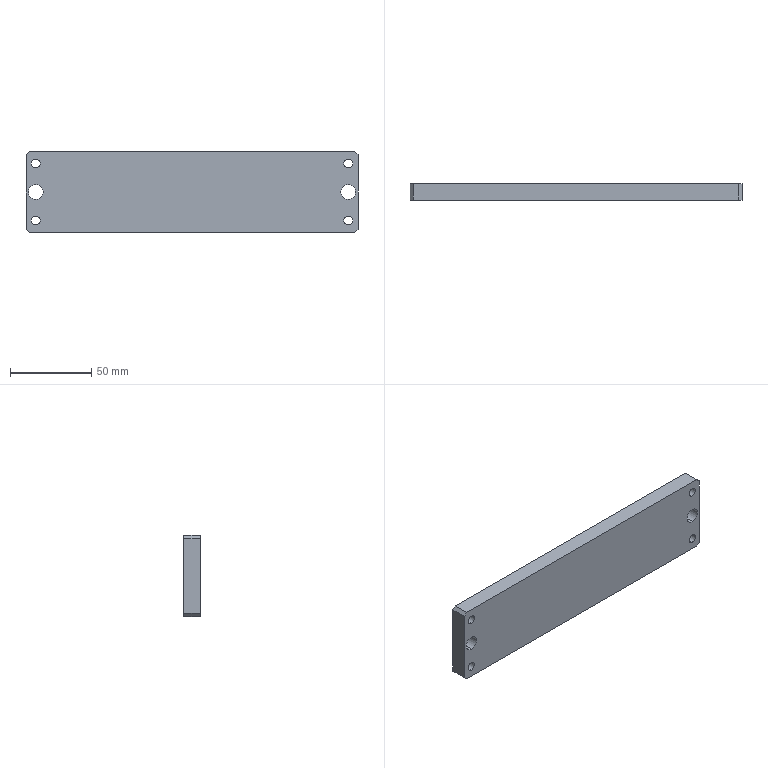Part | STEP file | MT-COMBO-119-S011 | 1 solid | 34 faces | box 204 x 10 x 50 mm | volume 98448 mm3 | cylinder 20 | plane 14 | commonest cylinder face diameters 5.5 x8 10 x8 9 x4
STEP:
#1=CARTESIAN_POINT('',(96.,-5.,-4.5));
#2=VERTEX_POINT('',#1);
#3=CARTESIAN_POINT('',(96.,-5.,4.5));
#4=VERTEX_POINT('',#3);
#5=CARTESIAN_POINT('',(96.,-5.,0.));
#6=DIRECTION('',(0.,-1.,0.));
#7=DIRECTION('',(0.,0.,-1.));
#8=AXIS2_PLACEMENT_3D('',#5,#6,#7);
#9=CIRCLE('',#8,4.5);
#10=EDGE_CURVE('',#2,#4,#9,.T.);
#11=ORIENTED_EDGE('',*,*,#10,.T.);
#12=CARTESIAN_POINT('',(96.,5.,4.5));
#13=VERTEX_POINT('',#12);
#14=CARTESIAN_POINT('',(96.,5.,4.5));
#15=DIRECTION('',(0.,1.,0.));
#16=VECTOR('',#15,1000.);
#17=LINE('',#14,#16);
#18=EDGE_CURVE('',#4,#13,#17,.T.);
#19=ORIENTED_EDGE('',*,*,#18,.T.);
#20=CARTESIAN_POINT('',(96.,5.,-4.5));
#21=VERTEX_POINT('',#20);
#22=CARTESIAN_POINT('',(96.,5.,0.));
#23=DIRECTION('',(0.,-1.,0.));
#24=DIRECTION('',(0.,0.,-1.));
#25=AXIS2_PLACEMENT_3D('',#22,#23,#24);
#26=CIRCLE('',#25,4.5);
#27=EDGE_CURVE('',#21,#13,#26,.T.);
#28=ORIENTED_EDGE('',*,*,#27,.F.);
#29=CARTESIAN_POINT('',(96.,5.,-4.5));
#30=DIRECTION('',(0.,1.,0.));
#31=VECTOR('',#30,1000.);
#32=LINE('',#29,#31);
#33=EDGE_CURVE('',#2,#21,#32,.T.);
#34=ORIENTED_EDGE('',*,*,#33,.F.);
#35=EDGE_LOOP('',(#11,#19,#28,#34));
#36=FACE_OUTER_BOUND('',#35,.T.);
#37=CARTESIAN_POINT('',(96.,5.,0.));
#38=DIRECTION('',(0.,1.,0.));
#39=DIRECTION('',(0.,0.,-1.));
#40=AXIS2_PLACEMENT_3D('',#37,#38,#39);
#41=CYLINDRICAL_SURFACE('',#40,4.5);
#42=ADVANCED_FACE('',(#36),#41,.F.);
#43=CARTESIAN_POINT('',(-96.,-5.,-4.5));
#44=VERTEX_POINT('',#43);
#45=CARTESIAN_POINT('',(-96.,-5.,4.5));
#46=VERTEX_POINT('',#45);
#47=CARTESIAN_POINT('',(-96.,-5.,0.));
#48=DIRECTION('',(0.,-1.,0.));
#49=DIRECTION('',(0.,0.,-1.));
#50=AXIS2_PLACEMENT_3D('',#47,#48,#49);
#51=CIRCLE('',#50,4.5);
#52=EDGE_CURVE('',#44,#46,#51,.T.);
#53=ORIENTED_EDGE('',*,*,#52,.T.);
#54=CARTESIAN_POINT('',(-96.,5.,4.5));
#55=VERTEX_POINT('',#54);
#56=CARTESIAN_POINT('',(-96.,5.,4.5));
#57=DIRECTION('',(0.,1.,0.));
#58=VECTOR('',#57,1000.);
#59=LINE('',#56,#58);
#60=EDGE_CURVE('',#46,#55,#59,.T.);
#61=ORIENTED_EDGE('',*,*,#60,.T.);
#62=CARTESIAN_POINT('',(-96.,5.,-4.5));
#63=VERTEX_POINT('',#62);
#64=CARTESIAN_POINT('',(-96.,5.,0.));
#65=DIRECTION('',(0.,-1.,0.));
#66=DIRECTION('',(0.,0.,-1.));
#67=AXIS2_PLACEMENT_3D('',#64,#65,#66);
#68=CIRCLE('',#67,4.5);
#69=EDGE_CURVE('',#63,#55,#68,.T.);
#70=ORIENTED_EDGE('',*,*,#69,.F.);
#71=CARTESIAN_POINT('',(-96.,5.,-4.5));
#72=DIRECTION('',(0.,1.,0.));
#73=VECTOR('',#72,1000.);
#74=LINE('',#71,#73);
#75=EDGE_CURVE('',#44,#63,#74,.T.);
#76=ORIENTED_EDGE('',*,*,#75,.F.);
#77=EDGE_LOOP('',(#53,#61,#70,#76));
#78=FACE_OUTER_BOUND('',#77,.T.);
#79=CARTESIAN_POINT('',(-96.,5.,0.));
#80=DIRECTION('',(0.,1.,0.));
#81=DIRECTION('',(0.,0.,-1.));
#82=AXIS2_PLACEMENT_3D('',#79,#80,#81);
#83=CYLINDRICAL_SURFACE('',#82,4.5);
#84=ADVANCED_FACE('',(#78),#83,.F.);
#85=CARTESIAN_POINT('',(-96.,-0.7,12.5));
#86=VERTEX_POINT('',#85);
#87=CARTESIAN_POINT('',(-96.,-0.7,22.5));
#88=VERTEX_POINT('',#87);
#89=CARTESIAN_POINT('',(-96.,-0.7,17.5));
#90=DIRECTION('',(0.,-1.,0.));
#91=DIRECTION('',(0.,0.,-1.));
#92=AXIS2_PLACEMENT_3D('',#89,#90,#91);
#93=CIRCLE('',#92,5.);
#94=EDGE_CURVE('',#86,#88,#93,.T.);
#95=ORIENTED_EDGE('',*,*,#94,.T.);
#96=CARTESIAN_POINT('',(-96.,5.,22.5));
#97=VERTEX_POINT('',#96);
#98=CARTESIAN_POINT('',(-96.,5.,22.5));
#99=DIRECTION('',(0.,1.,0.));
#100=VECTOR('',#99,1000.);
#101=LINE('',#98,#100);
#102=EDGE_CURVE('',#88,#97,#101,.T.);
#103=ORIENTED_EDGE('',*,*,#102,.T.);
#104=CARTESIAN_POINT('',(-96.,5.,12.5));
#105=VERTEX_POINT('',#104);
#106=CARTESIAN_POINT('',(-96.,5.,17.5));
#107=DIRECTION('',(0.,-1.,0.));
#108=DIRECTION('',(0.,0.,-1.));
#109=AXIS2_PLACEMENT_3D('',#106,#107,#108);
#110=CIRCLE('',#109,5.);
#111=EDGE_CURVE('',#105,#97,#110,.T.);
#112=ORIENTED_EDGE('',*,*,#111,.F.);
#113=CARTESIAN_POINT('',(-96.,5.,12.5));
#114=DIRECTION('',(0.,1.,0.));
#115=VECTOR('',#114,1000.);
#116=LINE('',#113,#115);
#117=EDGE_CURVE('',#86,#105,#116,.T.);
#118=ORIENTED_EDGE('',*,*,#117,.F.);
#119=EDGE_LOOP('',(#95,#103,#112,#118));
#120=FACE_OUTER_BOUND('',#119,.T.);
#121=CARTESIAN_POINT('',(-96.,5.,17.5));
#122=DIRECTION('',(0.,1.,0.));
#123=DIRECTION('',(0.,0.,-1.));
#124=AXIS2_PLACEMENT_3D('',#121,#122,#123);
#125=CYLINDRICAL_SURFACE('',#124,5.);
#126=ADVANCED_FACE('',(#120),#125,.F.);
#127=CARTESIAN_POINT('',(-96.,-5.,14.75));
#128=VERTEX_POINT('',#127);
#129=CARTESIAN_POINT('',(-96.,-5.,20.25));
#130=VERTEX_POINT('',#129);
#131=CARTESIAN_POINT('',(-96.,-5.,17.5));
#132=DIRECTION('',(0.,-1.,0.));
#133=DIRECTION('',(0.,0.,-1.));
#134=AXIS2_PLACEMENT_3D('',#131,#132,#133);
#135=CIRCLE('',#134,2.75);
#136=EDGE_CURVE('',#128,#130,#135,.T.);
#137=ORIENTED_EDGE('',*,*,#136,.T.);
#138=CARTESIAN_POINT('',(-96.,-0.7,20.25));
#139=VERTEX_POINT('',#138);
#140=CARTESIAN_POINT('',(-96.,5.,20.25));
#141=DIRECTION('',(0.,1.,0.));
#142=VECTOR('',#141,1000.);
#143=LINE('',#140,#142);
#144=EDGE_CURVE('',#130,#139,#143,.T.);
#145=ORIENTED_EDGE('',*,*,#144,.T.);
#146=CARTESIAN_POINT('',(-96.,-0.7,14.75));
#147=VERTEX_POINT('',#146);
#148=CARTESIAN_POINT('',(-96.,-0.7,17.5));
#149=DIRECTION('',(0.,-1.,0.));
#150=DIRECTION('',(0.,0.,-1.));
#151=AXIS2_PLACEMENT_3D('',#148,#149,#150);
#152=CIRCLE('',#151,2.75);
#153=EDGE_CURVE('',#147,#139,#152,.T.);
#154=ORIENTED_EDGE('',*,*,#153,.F.);
#155=CARTESIAN_POINT('',(-96.,5.,14.75));
#156=DIRECTION('',(0.,1.,0.));
#157=VECTOR('',#156,1000.);
#158=LINE('',#155,#157);
#159=EDGE_CURVE('',#128,#147,#158,.T.);
#160=ORIENTED_EDGE('',*,*,#159,.F.);
#161=EDGE_LOOP('',(#137,#145,#154,#160));
#162=FACE_OUTER_BOUND('',#161,.T.);
#163=CARTESIAN_POINT('',(-96.,5.,17.5));
#164=DIRECTION('',(0.,1.,0.));
#165=DIRECTION('',(0.,0.,-1.));
#166=AXIS2_PLACEMENT_3D('',#163,#164,#165);
#167=CYLINDRICAL_SURFACE('',#166,2.75);
#168=ADVANCED_FACE('',(#162),#167,.F.);
#169=CARTESIAN_POINT('',(-96.,-0.7,-22.5));
#170=VERTEX_POINT('',#169);
#171=CARTESIAN_POINT('',(-96.,-0.7,-12.5));
#172=VERTEX_POINT('',#171);
#173=CARTESIAN_POINT('',(-96.,-0.7,-17.5));
#174=DIRECTION('',(0.,-1.,0.));
#175=DIRECTION('',(0.,0.,-1.));
#176=AXIS2_PLACEMENT_3D('',#173,#174,#175);
#177=CIRCLE('',#176,5.);
#178=EDGE_CURVE('',#170,#172,#177,.T.);
#179=ORIENTED_EDGE('',*,*,#178,.T.);
#180=CARTESIAN_POINT('',(-96.,5.,-12.5));
#181=VERTEX_POINT('',#180);
#182=CARTESIAN_POINT('',(-96.,5.,-12.5));
#183=DIRECTION('',(0.,1.,0.));
#184=VECTOR('',#183,1000.);
#185=LINE('',#182,#184);
#186=EDGE_CURVE('',#172,#181,#185,.T.);
#187=ORIENTED_EDGE('',*,*,#186,.T.);
#188=CARTESIAN_POINT('',(-96.,5.,-22.5));
#189=VERTEX_POINT('',#188);
#190=CARTESIAN_POINT('',(-96.,5.,-17.5));
#191=DIRECTION('',(0.,-1.,0.));
#192=DIRECTION('',(0.,0.,-1.));
#193=AXIS2_PLACEMENT_3D('',#190,#191,#192);
#194=CIRCLE('',#193,5.);
#195=EDGE_CURVE('',#189,#181,#194,.T.);
#196=ORIENTED_EDGE('',*,*,#195,.F.);
#197=CARTESIAN_POINT('',(-96.,5.,-22.5));
#198=DIRECTION('',(0.,1.,0.));
#199=VECTOR('',#198,1000.);
#200=LINE('',#197,#199);
#201=EDGE_CURVE('',#170,#189,#200,.T.);
#202=ORIENTED_EDGE('',*,*,#201,.F.);
#203=EDGE_LOOP('',(#179,#187,#196,#202));
#204=FACE_OUTER_BOUND('',#203,.T.);
#205=CARTESIAN_POINT('',(-96.,5.,-17.5));
#206=DIRECTION('',(0.,1.,0.));
#207=DIRECTION('',(0.,0.,-1.));
#208=AXIS2_PLACEMENT_3D('',#205,#206,#207);
#209=CYLINDRICAL_SURFACE('',#208,5.);
#210=ADVANCED_FACE('',(#204),#209,.F.);
#211=CARTESIAN_POINT('',(-96.,-5.,-20.25));
#212=VERTEX_POINT('',#211);
#213=CARTESIAN_POINT('',(-96.,-5.,-14.75));
#214=VERTEX_POINT('',#213);
#215=CARTESIAN_POINT('',(-96.,-5.,-17.5));
#216=DIRECTION('',(0.,-1.,0.));
#217=DIRECTION('',(0.,0.,-1.));
#218=AXIS2_PLACEMENT_3D('',#215,#216,#217);
#219=CIRCLE('',#218,2.75);
#220=EDGE_CURVE('',#212,#214,#219,.T.);
#221=ORIENTED_EDGE('',*,*,#220,.T.);
#222=CARTESIAN_POINT('',(-96.,-0.7,-14.75));
#223=VERTEX_POINT('',#222);
#224=CARTESIAN_POINT('',(-96.,5.,-14.75));
#225=DIRECTION('',(0.,1.,0.));
#226=VECTOR('',#225,1000.);
#227=LINE('',#224,#226);
#228=EDGE_CURVE('',#214,#223,#227,.T.);
#229=ORIENTED_EDGE('',*,*,#228,.T.);
#230=CARTESIAN_POINT('',(-96.,-0.7,-20.25));
#231=VERTEX_POINT('',#230);
#232=CARTESIAN_POINT('',(-96.,-0.7,-17.5));
#233=DIRECTION('',(0.,-1.,0.));
#234=DIRECTION('',(0.,0.,-1.));
#235=AXIS2_PLACEMENT_3D('',#232,#233,#234);
#236=CIRCLE('',#235,2.75);
#237=EDGE_CURVE('',#231,#223,#236,.T.);
#238=ORIENTED_EDGE('',*,*,#237,.F.);
#239=CARTESIAN_POINT('',(-96.,5.,-20.25));
#240=DIRECTION('',(0.,1.,0.));
#241=VECTOR('',#240,1000.);
#242=LINE('',#239,#241);
#243=EDGE_CURVE('',#212,#231,#242,.T.);
#244=ORIENTED_EDGE('',*,*,#243,.F.);
#245=EDGE_LOOP('',(#221,#229,#238,#244));
#246=FACE_OUTER_BOUND('',#245,.T.);
#247=CARTESIAN_POINT('',(-96.,5.,-17.5));
#248=DIRECTION('',(0.,1.,0.));
#249=DIRECTION('',(0.,0.,-1.));
#250=AXIS2_PLACEMENT_3D('',#247,#248,#249);
#251=CYLINDRICAL_SURFACE('',#250,2.75);
#252=ADVANCED_FACE('',(#246),#251,.F.);
#253=CARTESIAN_POINT('',(96.,-0.7,-22.5));
#254=VERTEX_POINT('',#253);
#255=CARTESIAN_POINT('',(96.,-0.7,-12.5));
#256=VERTEX_POINT('',#255);
#257=CARTESIAN_POINT('',(96.,-0.7,-17.5));
#258=DIRECTION('',(0.,-1.,0.));
#259=DIRECTION('',(0.,0.,-1.));
#260=AXIS2_PLACEMENT_3D('',#257,#258,#259);
#261=CIRCLE('',#260,5.);
#262=EDGE_CURVE('',#254,#256,#261,.T.);
#263=ORIENTED_EDGE('',*,*,#262,.T.);
#264=CARTESIAN_POINT('',(96.,5.,-12.5));
#265=VERTEX_POINT('',#264);
#266=CARTESIAN_POINT('',(96.,5.,-12.5));
#267=DIRECTION('',(0.,1.,0.));
#268=VECTOR('',#267,1000.);
#269=LINE('',#266,#268);
#270=EDGE_CURVE('',#256,#265,#269,.T.);
#271=ORIENTED_EDGE('',*,*,#270,.T.);
#272=CARTESIAN_POINT('',(96.,5.,-22.5));
#273=VERTEX_POINT('',#272);
#274=CARTESIAN_POINT('',(96.,5.,-17.5));
#275=DIRECTION('',(0.,-1.,0.));
#276=DIRECTION('',(0.,0.,-1.));
#277=AXIS2_PLACEMENT_3D('',#274,#275,#276);
#278=CIRCLE('',#277,5.);
#279=EDGE_CURVE('',#273,#265,#278,.T.);
#280=ORIENTED_EDGE('',*,*,#279,.F.);
#281=CARTESIAN_POINT('',(96.,5.,-22.5));
#282=DIRECTION('',(0.,1.,0.));
#283=VECTOR('',#282,1000.);
#284=LINE('',#281,#283);
#285=EDGE_CURVE('',#254,#273,#284,.T.);
#286=ORIENTED_EDGE('',*,*,#285,.F.);
#287=EDGE_LOOP('',(#263,#271,#280,#286));
#288=FACE_OUTER_BOUND('',#287,.T.);
#289=CARTESIAN_POINT('',(96.,5.,-17.5));
#290=DIRECTION('',(0.,1.,0.));
#291=DIRECTION('',(0.,0.,-1.));
#292=AXIS2_PLACEMENT_3D('',#289,#290,#291);
#293=CYLINDRICAL_SURFACE('',#292,5.);
#294=ADVANCED_FACE('',(#288),#293,.F.);
#295=CARTESIAN_POINT('',(96.,-5.,-20.25));
#296=VERTEX_POINT('',#295);
#297=CARTESIAN_POINT('',(96.,-5.,-14.75));
#298=VERTEX_POINT('',#297);
#299=CARTESIAN_POINT('',(96.,-5.,-17.5));
#300=DIRECTION('',(0.,-1.,0.));
#301=DIRECTION('',(0.,0.,-1.));
#302=AXIS2_PLACEMENT_3D('',#299,#300,#301);
#303=CIRCLE('',#302,2.75);
#304=EDGE_CURVE('',#296,#298,#303,.T.);
#305=ORIENTED_EDGE('',*,*,#304,.T.);
#306=CARTESIAN_POINT('',(96.,-0.7,-14.75));
#307=VERTEX_POINT('',#306);
#308=CARTESIAN_POINT('',(96.,5.,-14.75));
#309=DIRECTION('',(0.,1.,0.));
#310=VECTOR('',#309,1000.);
#311=LINE('',#308,#310);
#312=EDGE_CURVE('',#298,#307,#311,.T.);
#313=ORIENTED_EDGE('',*,*,#312,.T.);
#314=CARTESIAN_POINT('',(96.,-0.7,-20.25));
#315=VERTEX_POINT('',#314);
#316=CARTESIAN_POINT('',(96.,-0.7,-17.5));
#317=DIRECTION('',(0.,-1.,0.));
#318=DIRECTION('',(0.,0.,-1.));
#319=AXIS2_PLACEMENT_3D('',#316,#317,#318);
#320=CIRCLE('',#319,2.75);
#321=EDGE_CURVE('',#315,#307,#320,.T.);
#322=ORIENTED_EDGE('',*,*,#321,.F.);
#323=CARTESIAN_POINT('',(96.,5.,-20.25));
#324=DIRECTION('',(0.,1.,0.));
#325=VECTOR('',#324,1000.);
#326=LINE('',#323,#325);
#327=EDGE_CURVE('',#296,#315,#326,.T.);
#328=ORIENTED_EDGE('',*,*,#327,.F.);
#329=EDGE_LOOP('',(#305,#313,#322,#328));
#330=FACE_OUTER_BOUND('',#329,.T.);
#331=CARTESIAN_POINT('',(96.,5.,-17.5));
#332=DIRECTION('',(0.,1.,0.));
#333=DIRECTION('',(0.,0.,-1.));
#334=AXIS2_PLACEMENT_3D('',#331,#332,#333);
#335=CYLINDRICAL_SURFACE('',#334,2.75);
#336=ADVANCED_FACE('',(#330),#335,.F.);
#337=CARTESIAN_POINT('',(96.,-0.7,12.5));
#338=VERTEX_POINT('',#337);
#339=CARTESIAN_POINT('',(96.,-0.7,22.5));
#340=VERTEX_POINT('',#339);
#341=CARTESIAN_POINT('',(96.,-0.7,17.5));
#342=DIRECTION('',(0.,-1.,0.));
#343=DIRECTION('',(0.,0.,-1.));
#344=AXIS2_PLACEMENT_3D('',#341,#342,#343);
#345=CIRCLE('',#344,5.);
#346=EDGE_CURVE('',#338,#340,#345,.T.);
#347=ORIENTED_EDGE('',*,*,#346,.T.);
#348=CARTESIAN_POINT('',(96.,5.,22.5));
#349=VERTEX_POINT('',#348);
#350=CARTESIAN_POINT('',(96.,5.,22.5));
#351=DIRECTION('',(0.,1.,0.));
#352=VECTOR('',#351,1000.);
#353=LINE('',#350,#352);
#354=EDGE_CURVE('',#340,#349,#353,.T.);
#355=ORIENTED_EDGE('',*,*,#354,.T.);
#356=CARTESIAN_POINT('',(96.,5.,12.5));
#357=VERTEX_POINT('',#356);
#358=CARTESIAN_POINT('',(96.,5.,17.5));
#359=DIRECTION('',(0.,-1.,0.));
#360=DIRECTION('',(0.,0.,-1.));
#361=AXIS2_PLACEMENT_3D('',#358,#359,#360);
#362=CIRCLE('',#361,5.);
#363=EDGE_CURVE('',#357,#349,#362,.T.);
#364=ORIENTED_EDGE('',*,*,#363,.F.);
#365=CARTESIAN_POINT('',(96.,5.,12.5));
#366=DIRECTION('',(0.,1.,0.));
#367=VECTOR('',#366,1000.);
#368=LINE('',#365,#367);
#369=EDGE_CURVE('',#338,#357,#368,.T.);
#370=ORIENTED_EDGE('',*,*,#369,.F.);
#371=EDGE_LOOP('',(#347,#355,#364,#370));
#372=FACE_OUTER_BOUND('',#371,.T.);
#373=CARTESIAN_POINT('',(96.,5.,17.5));
#374=DIRECTION('',(0.,1.,0.));
#375=DIRECTION('',(0.,0.,-1.));
#376=AXIS2_PLACEMENT_3D('',#373,#374,#375);
#377=CYLINDRICAL_SURFACE('',#376,5.);
#378=ADVANCED_FACE('',(#372),#377,.F.);
#379=CARTESIAN_POINT('',(96.,-5.,14.75));
#380=VERTEX_POINT('',#379);
#381=CARTESIAN_POINT('',(96.,-5.,20.25));
#382=VERTEX_POINT('',#381);
#383=CARTESIAN_POINT('',(96.,-5.,17.5));
#384=DIRECTION('',(0.,-1.,0.));
#385=DIRECTION('',(0.,0.,-1.));
#386=AXIS2_PLACEMENT_3D('',#383,#384,#385);
#387=CIRCLE('',#386,2.75);
#388=EDGE_CURVE('',#380,#382,#387,.T.);
#389=ORIENTED_EDGE('',*,*,#388,.T.);
#390=CARTESIAN_POINT('',(96.,-0.7,20.25));
#391=VERTEX_POINT('',#390);
#392=CARTESIAN_POINT('',(96.,5.,20.25));
#393=DIRECTION('',(0.,1.,0.));
#394=VECTOR('',#393,1000.);
#395=LINE('',#392,#394);
#396=EDGE_CURVE('',#382,#391,#395,.T.);
#397=ORIENTED_EDGE('',*,*,#396,.T.);
#398=CARTESIAN_POINT('',(96.,-0.7,14.75));
#399=VERTEX_POINT('',#398);
#400=CARTESIAN_POINT('',(96.,-0.7,17.5));
#401=DIRECTION('',(0.,-1.,0.));
#402=DIRECTION('',(0.,0.,-1.));
#403=AXIS2_PLACEMENT_3D('',#400,#401,#402);
#404=CIRCLE('',#403,2.75);
#405=EDGE_CURVE('',#399,#391,#404,.T.);
#406=ORIENTED_EDGE('',*,*,#405,.F.);
#407=CARTESIAN_POINT('',(96.,5.,14.75));
#408=DIRECTION('',(0.,1.,0.));
#409=VECTOR('',#408,1000.);
#410=LINE('',#407,#409);
#411=EDGE_CURVE('',#380,#399,#410,.T.);
#412=ORIENTED_EDGE('',*,*,#411,.F.);
#413=EDGE_LOOP('',(#389,#397,#406,#412));
#414=FACE_OUTER_BOUND('',#413,.T.);
#415=CARTESIAN_POINT('',(96.,5.,17.5));
#416=DIRECTION('',(0.,1.,0.));
#417=DIRECTION('',(0.,0.,-1.));
#418=AXIS2_PLACEMENT_3D('',#415,#416,#417);
#419=CYLINDRICAL_SURFACE('',#418,2.75);
#420=ADVANCED_FACE('',(#414),#419,.F.);
#421=CARTESIAN_POINT('',(102.,-5.,-23.));
#422=VERTEX_POINT('',#421);
#423=CARTESIAN_POINT('',(102.,-5.,23.));
#424=VERTEX_POINT('',#423);
#425=CARTESIAN_POINT('',(102.,-5.,25.));
#426=DIRECTION('',(0.,0.,1.));
#427=VECTOR('',#426,1000.);
#428=LINE('',#425,#427);
#429=EDGE_CURVE('',#422,#424,#428,.T.);
#430=ORIENTED_EDGE('',*,*,#429,.F.);
#431=CARTESIAN_POINT('',(102.,5.,-23.));
#432=VERTEX_POINT('',#431);
#433=CARTESIAN_POINT('',(102.,5.,-23.));
#434=DIRECTION('',(0.,-1.,0.));
#435=VECTOR('',#434,1000.);
#436=LINE('',#433,#435);
#437=EDGE_CURVE('',#432,#422,#436,.T.);
#438=ORIENTED_EDGE('',*,*,#437,.F.);
#439=CARTESIAN_POINT('',(102.,5.,23.));
#440=VERTEX_POINT('',#439);
#441=CARTESIAN_POINT('',(102.,5.,25.));
#442=DIRECTION('',(0.,0.,1.));
#443=VECTOR('',#442,1000.);
#444=LINE('',#441,#443);
#445=EDGE_CURVE('',#432,#440,#444,.T.);
#446=ORIENTED_EDGE('',*,*,#445,.T.);
#447=CARTESIAN_POINT('',(102.,5.,23.));
#448=DIRECTION('',(0.,1.,0.));
#449=VECTOR('',#448,1000.);
#450=LINE('',#447,#449);
#451=EDGE_CURVE('',#424,#440,#450,.T.);
#452=ORIENTED_EDGE('',*,*,#451,.F.);
#453=EDGE_LOOP('',(#430,#438,#446,#452));
#454=FACE_OUTER_BOUND('',#453,.T.);
#455=CARTESIAN_POINT('',(102.,5.,25.));
#456=DIRECTION('',(-1.,0.,0.));
#457=DIRECTION('',(0.,0.,-1.));
#458=AXIS2_PLACEMENT_3D('',#455,#456,#457);
#459=PLANE('',#458);
#460=ADVANCED_FACE('',(#454),#459,.F.);
#461=CARTESIAN_POINT('',(100.,5.,25.));
#462=VERTEX_POINT('',#461);
#463=CARTESIAN_POINT('',(-100.,5.,25.));
#464=VERTEX_POINT('',#463);
#465=CARTESIAN_POINT('',(-154.5,5.,25.));
#466=DIRECTION('',(-1.,0.,0.));
#467=VECTOR('',#466,1000.);
#468=LINE('',#465,#467);
#469=EDGE_CURVE('',#462,#464,#468,.T.);
#470=ORIENTED_EDGE('',*,*,#469,.T.);
#471=CARTESIAN_POINT('',(-100.,-5.,25.));
#472=VERTEX_POINT('',#471);
#473=CARTESIAN_POINT('',(-100.,5.,25.));
#474=DIRECTION('',(0.,1.,0.));
#475=VECTOR('',#474,1000.);
#476=LINE('',#473,#475);
#477=EDGE_CURVE('',#472,#464,#476,.T.);
#478=ORIENTED_EDGE('',*,*,#477,.F.);
#479=CARTESIAN_POINT('',(100.,-5.,25.));
#480=VERTEX_POINT('',#479);
#481=CARTESIAN_POINT('',(-154.5,-5.,25.));
#482=DIRECTION('',(-1.,0.,0.));
#483=VECTOR('',#482,1000.);
#484=LINE('',#481,#483);
#485=EDGE_CURVE('',#480,#472,#484,.T.);
#486=ORIENTED_EDGE('',*,*,#485,.F.);
#487=CARTESIAN_POINT('',(100.,5.,25.));
#488=DIRECTION('',(0.,-1.,0.));
#489=VECTOR('',#488,1000.);
#490=LINE('',#487,#489);
#491=EDGE_CURVE('',#462,#480,#490,.T.);
#492=ORIENTED_EDGE('',*,*,#491,.F.);
#493=EDGE_LOOP('',(#470,#478,#486,#492));
#494=FACE_OUTER_BOUND('',#493,.T.);
#495=CARTESIAN_POINT('',(-154.5,5.,25.));
#496=DIRECTION('',(0.,0.,-1.));
#497=DIRECTION('',(1.,0.,0.));
#498=AXIS2_PLACEMENT_3D('',#495,#496,#497);
#499=PLANE('',#498);
#500=ADVANCED_FACE('',(#494),#499,.F.);
#501=CARTESIAN_POINT('',(-102.,5.,23.));
#502=VERTEX_POINT('',#501);
#503=CARTESIAN_POINT('',(-102.,5.,-23.));
#504=VERTEX_POINT('',#503);
#505=CARTESIAN_POINT('',(-102.,5.,25.));
#506=DIRECTION('',(0.,0.,-1.));
#507=VECTOR('',#506,1000.);
#508=LINE('',#505,#507);
#509=EDGE_CURVE('',#502,#504,#508,.T.);
#510=ORIENTED_EDGE('',*,*,#509,.T.);
#511=CARTESIAN_POINT('',(-102.,-5.,-23.));
#512=VERTEX_POINT('',#511);
#513=CARTESIAN_POINT('',(-102.,5.,-23.));
#514=DIRECTION('',(0.,1.,0.));
#515=VECTOR('',#514,1000.);
#516=LINE('',#513,#515);
#517=EDGE_CURVE('',#512,#504,#516,.T.);
#518=ORIENTED_EDGE('',*,*,#517,.F.);
#519=CARTESIAN_POINT('',(-102.,-5.,23.));
#520=VERTEX_POINT('',#519);
#521=CARTESIAN_POINT('',(-102.,-5.,25.));
#522=DIRECTION('',(0.,0.,-1.));
#523=VECTOR('',#522,1000.);
#524=LINE('',#521,#523);
#525=EDGE_CURVE('',#520,#512,#524,.T.);
#526=ORIENTED_EDGE('',*,*,#525,.F.);
#527=CARTESIAN_POINT('',(-102.,5.,23.));
#528=DIRECTION('',(0.,-1.,0.));
#529=VECTOR('',#528,1000.);
#530=LINE('',#527,#529);
#531=EDGE_CURVE('',#502,#520,#530,.T.);
#532=ORIENTED_EDGE('',*,*,#531,.F.);
#533=EDGE_LOOP('',(#510,#518,#526,#532));
#534=FACE_OUTER_BOUND('',#533,.T.);
#535=CARTESIAN_POINT('',(-102.,5.,25.));
#536=DIRECTION('',(1.,0.,0.));
#537=DIRECTION('',(0.,0.,1.));
#538=AXIS2_PLACEMENT_3D('',#535,#536,#537);
#539=PLANE('',#538);
#540=ADVANCED_FACE('',(#534),#539,.F.);
#541=CARTESIAN_POINT('',(-100.,-5.,-25.));
#542=VERTEX_POINT('',#541);
#543=CARTESIAN_POINT('',(100.,-5.,-25.));
#544=VERTEX_POINT('',#543);
#545=CARTESIAN_POINT('',(-154.5,-5.,-25.));
#546=DIRECTION('',(1.,0.,0.));
#547=VECTOR('',#546,1000.);
#548=LINE('',#545,#547);
#549=EDGE_CURVE('',#542,#544,#548,.T.);
#550=ORIENTED_EDGE('',*,*,#549,.F.);
#551=CARTESIAN_POINT('',(-100.,5.,-25.));
#552=VERTEX_POINT('',#551);
#553=CARTESIAN_POINT('',(-100.,5.,-25.));
#554=DIRECTION('',(0.,-1.,0.));
#555=VECTOR('',#554,1000.);
#556=LINE('',#553,#555);
#557=EDGE_CURVE('',#552,#542,#556,.T.);
#558=ORIENTED_EDGE('',*,*,#557,.F.);
#559=CARTESIAN_POINT('',(100.,5.,-25.));
#560=VERTEX_POINT('',#559);
#561=CARTESIAN_POINT('',(-154.5,5.,-25.));
#562=DIRECTION('',(1.,0.,0.));
#563=VECTOR('',#562,1000.);
#564=LINE('',#561,#563);
#565=EDGE_CURVE('',#552,#560,#564,.T.);
#566=ORIENTED_EDGE('',*,*,#565,.T.);
#567=CARTESIAN_POINT('',(100.,5.,-25.));
#568=DIRECTION('',(0.,1.,0.));
#569=VECTOR('',#568,1000.);
#570=LINE('',#567,#569);
#571=EDGE_CURVE('',#544,#560,#570,.T.);
#572=ORIENTED_EDGE('',*,*,#571,.F.);
#573=EDGE_LOOP('',(#550,#558,#566,#572));
#574=FACE_OUTER_BOUND('',#573,.T.);
#575=CARTESIAN_POINT('',(-154.5,5.,-25.));
#576=DIRECTION('',(0.,0.,1.));
#577=DIRECTION('',(-1.,0.,0.));
#578=AXIS2_PLACEMENT_3D('',#575,#576,#577);
#579=PLANE('',#578);
#580=ADVANCED_FACE('',(#574),#579,.F.);
#581=ORIENTED_EDGE('',*,*,#27,.T.);
#582=CARTESIAN_POINT('',(96.,5.,0.));
#583=DIRECTION('',(0.,-1.,0.));
#584=DIRECTION('',(0.,0.,-1.));
#585=AXIS2_PLACEMENT_3D('',#582,#583,#584);
#586=CIRCLE('',#585,4.5);
#587=EDGE_CURVE('',#13,#21,#586,.T.);
#588=ORIENTED_EDGE('',*,*,#587,.T.);
#589=EDGE_LOOP('',(#581,#588));
#590=FACE_BOUND('',#589,.T.);
#591=ORIENTED_EDGE('',*,*,#69,.T.);
#592=CARTESIAN_POINT('',(-96.,5.,0.));
#593=DIRECTION('',(0.,-1.,0.));
#594=DIRECTION('',(0.,0.,-1.));
#595=AXIS2_PLACEMENT_3D('',#592,#593,#594);
#596=CIRCLE('',#595,4.5);
#597=EDGE_CURVE('',#55,#63,#596,.T.);
#598=ORIENTED_EDGE('',*,*,#597,.T.);
#599=EDGE_LOOP('',(#591,#598));
#600=FACE_BOUND('',#599,.T.);
#601=ORIENTED_EDGE('',*,*,#111,.T.);
#602=CARTESIAN_POINT('',(-96.,5.,17.5));
#603=DIRECTION('',(0.,-1.,0.));
#604=DIRECTION('',(0.,0.,-1.));
#605=AXIS2_PLACEMENT_3D('',#602,#603,#604);
#606=CIRCLE('',#605,5.);
#607=EDGE_CURVE('',#97,#105,#606,.T.);
#608=ORIENTED_EDGE('',*,*,#607,.T.);
#609=EDGE_LOOP('',(#601,#608));
#610=FACE_BOUND('',#609,.T.);
#611=ORIENTED_EDGE('',*,*,#195,.T.);
#612=CARTESIAN_POINT('',(-96.,5.,-17.5));
#613=DIRECTION('',(0.,-1.,0.));
#614=DIRECTION('',(0.,0.,-1.));
#615=AXIS2_PLACEMENT_3D('',#612,#613,#614);
#616=CIRCLE('',#615,5.);
#617=EDGE_CURVE('',#181,#189,#616,.T.);
#618=ORIENTED_EDGE('',*,*,#617,.T.);
#619=EDGE_LOOP('',(#611,#618));
#620=FACE_BOUND('',#619,.T.);
#621=ORIENTED_EDGE('',*,*,#279,.T.);
#622=CARTESIAN_POINT('',(96.,5.,-17.5));
#623=DIRECTION('',(0.,-1.,0.));
#624=DIRECTION('',(0.,0.,-1.));
#625=AXIS2_PLACEMENT_3D('',#622,#623,#624);
#626=CIRCLE('',#625,5.);
#627=EDGE_CURVE('',#265,#273,#626,.T.);
#628=ORIENTED_EDGE('',*,*,#627,.T.);
#629=EDGE_LOOP('',(#621,#628));
#630=FACE_BOUND('',#629,.T.);
#631=ORIENTED_EDGE('',*,*,#363,.T.);
#632=CARTESIAN_POINT('',(96.,5.,17.5));
#633=DIRECTION('',(0.,-1.,0.));
#634=DIRECTION('',(0.,0.,-1.));
#635=AXIS2_PLACEMENT_3D('',#632,#633,#634);
#636=CIRCLE('',#635,5.);
#637=EDGE_CURVE('',#349,#357,#636,.T.);
#638=ORIENTED_EDGE('',*,*,#637,.T.);
#639=EDGE_LOOP('',(#631,#638));
#640=FACE_BOUND('',#639,.T.);
#641=ORIENTED_EDGE('',*,*,#445,.F.);
#642=CARTESIAN_POINT('',(36.25,5.,-88.75));
#643=DIRECTION('',(0.7071,0.,0.7071));
#644=VECTOR('',#643,1000.);
#645=LINE('',#642,#644);
#646=EDGE_CURVE('',#560,#432,#645,.T.);
#647=ORIENTED_EDGE('',*,*,#646,.F.);
#648=ORIENTED_EDGE('',*,*,#565,.F.);
#649=CARTESIAN_POINT('',(-36.25,5.,-88.75));
#650=DIRECTION('',(0.7071,0.,-0.7071));
#651=VECTOR('',#650,1000.);
#652=LINE('',#649,#651);
#653=EDGE_CURVE('',#504,#552,#652,.T.);
#654=ORIENTED_EDGE('',*,*,#653,.F.);
#655=ORIENTED_EDGE('',*,*,#509,.F.);
#656=CARTESIAN_POINT('',(-36.25,5.,88.75));
#657=DIRECTION('',(-0.7071,0.,-0.7071));
#658=VECTOR('',#657,1000.);
#659=LINE('',#656,#658);
#660=EDGE_CURVE('',#464,#502,#659,.T.);
#661=ORIENTED_EDGE('',*,*,#660,.F.);
#662=ORIENTED_EDGE('',*,*,#469,.F.);
#663=CARTESIAN_POINT('',(36.25,5.,88.75));
#664=DIRECTION('',(-0.7071,0.,0.7071));
#665=VECTOR('',#664,1000.);
#666=LINE('',#663,#665);
#667=EDGE_CURVE('',#440,#462,#666,.T.);
#668=ORIENTED_EDGE('',*,*,#667,.F.);
#669=EDGE_LOOP('',(#641,#647,#648,#654,#655,#661,#662,#668));
#670=FACE_OUTER_BOUND('',#669,.T.);
#671=CARTESIAN_POINT('',(0.,5.,0.));
#672=DIRECTION('',(0.,1.,0.));
#673=DIRECTION('',(0.,0.,-1.));
#674=AXIS2_PLACEMENT_3D('',#671,#672,#673);
#675=PLANE('',#674);
#676=ADVANCED_FACE('',(#590,#600,#610,#620,#630,#640,#670),#675,.T.);
#677=ORIENTED_EDGE('',*,*,#10,.F.);
#678=CARTESIAN_POINT('',(96.,-5.,0.));
#679=DIRECTION('',(0.,-1.,0.));
#680=DIRECTION('',(0.,0.,-1.));
#681=AXIS2_PLACEMENT_3D('',#678,#679,#680);
#682=CIRCLE('',#681,4.5);
#683=EDGE_CURVE('',#4,#2,#682,.T.);
#684=ORIENTED_EDGE('',*,*,#683,.F.);
#685=EDGE_LOOP('',(#677,#684));
#686=FACE_BOUND('',#685,.T.);
#687=ORIENTED_EDGE('',*,*,#52,.F.);
#688=CARTESIAN_POINT('',(-96.,-5.,0.));
#689=DIRECTION('',(0.,-1.,0.));
#690=DIRECTION('',(0.,0.,-1.));
#691=AXIS2_PLACEMENT_3D('',#688,#689,#690);
#692=CIRCLE('',#691,4.5);
#693=EDGE_CURVE('',#46,#44,#692,.T.);
#694=ORIENTED_EDGE('',*,*,#693,.F.);
#695=EDGE_LOOP('',(#687,#694));
#696=FACE_BOUND('',#695,.T.);
#697=ORIENTED_EDGE('',*,*,#136,.F.);
#698=CARTESIAN_POINT('',(-96.,-5.,17.5));
#699=DIRECTION('',(0.,-1.,0.));
#700=DIRECTION('',(0.,0.,-1.));
#701=AXIS2_PLACEMENT_3D('',#698,#699,#700);
#702=CIRCLE('',#701,2.75);
#703=EDGE_CURVE('',#130,#128,#702,.T.);
#704=ORIENTED_EDGE('',*,*,#703,.F.);
#705=EDGE_LOOP('',(#697,#704));
#706=FACE_BOUND('',#705,.T.);
#707=ORIENTED_EDGE('',*,*,#220,.F.);
#708=CARTESIAN_POINT('',(-96.,-5.,-17.5));
#709=DIRECTION('',(0.,-1.,0.));
#710=DIRECTION('',(0.,0.,-1.));
#711=AXIS2_PLACEMENT_3D('',#708,#709,#710);
#712=CIRCLE('',#711,2.75);
#713=EDGE_CURVE('',#214,#212,#712,.T.);
#714=ORIENTED_EDGE('',*,*,#713,.F.);
#715=EDGE_LOOP('',(#707,#714));
#716=FACE_BOUND('',#715,.T.);
#717=ORIENTED_EDGE('',*,*,#304,.F.);
#718=CARTESIAN_POINT('',(96.,-5.,-17.5));
#719=DIRECTION('',(0.,-1.,0.));
#720=DIRECTION('',(0.,0.,-1.));
#721=AXIS2_PLACEMENT_3D('',#718,#719,#720);
#722=CIRCLE('',#721,2.75);
#723=EDGE_CURVE('',#298,#296,#722,.T.);
#724=ORIENTED_EDGE('',*,*,#723,.F.);
#725=EDGE_LOOP('',(#717,#724));
#726=FACE_BOUND('',#725,.T.);
#727=ORIENTED_EDGE('',*,*,#388,.F.);
#728=CARTESIAN_POINT('',(96.,-5.,17.5));
#729=DIRECTION('',(0.,-1.,0.));
#730=DIRECTION('',(0.,0.,-1.));
#731=AXIS2_PLACEMENT_3D('',#728,#729,#730);
#732=CIRCLE('',#731,2.75);
#733=EDGE_CURVE('',#382,#380,#732,.T.);
#734=ORIENTED_EDGE('',*,*,#733,.F.);
#735=EDGE_LOOP('',(#727,#734));
#736=FACE_BOUND('',#735,.T.);
#737=ORIENTED_EDGE('',*,*,#485,.T.);
#738=CARTESIAN_POINT('',(-102.,-5.,23.));
#739=DIRECTION('',(0.7071,0.,0.7071));
#740=VECTOR('',#739,1000.);
#741=LINE('',#738,#740);
#742=EDGE_CURVE('',#520,#472,#741,.T.);
#743=ORIENTED_EDGE('',*,*,#742,.F.);
#744=ORIENTED_EDGE('',*,*,#525,.T.);
#745=CARTESIAN_POINT('',(-100.,-5.,-25.));
#746=DIRECTION('',(-0.7071,0.,0.7071));
#747=VECTOR('',#746,1000.);
#748=LINE('',#745,#747);
#749=EDGE_CURVE('',#542,#512,#748,.T.);
#750=ORIENTED_EDGE('',*,*,#749,.F.);
#751=ORIENTED_EDGE('',*,*,#549,.T.);
#752=CARTESIAN_POINT('',(102.,-5.,-23.));
#753=DIRECTION('',(-0.7071,0.,-0.7071));
#754=VECTOR('',#753,1000.);
#755=LINE('',#752,#754);
#756=EDGE_CURVE('',#422,#544,#755,.T.);
#757=ORIENTED_EDGE('',*,*,#756,.F.);
#758=ORIENTED_EDGE('',*,*,#429,.T.);
#759=CARTESIAN_POINT('',(100.,-5.,25.));
#760=DIRECTION('',(0.7071,0.,-0.7071));
#761=VECTOR('',#760,1000.);
#762=LINE('',#759,#761);
#763=EDGE_CURVE('',#480,#424,#762,.T.);
#764=ORIENTED_EDGE('',*,*,#763,.F.);
#765=EDGE_LOOP('',(#737,#743,#744,#750,#751,#757,#758,#764));
#766=FACE_OUTER_BOUND('',#765,.T.);
#767=CARTESIAN_POINT('',(0.,-5.,0.));
#768=DIRECTION('',(0.,1.,0.));
#769=DIRECTION('',(0.,0.,-1.));
#770=AXIS2_PLACEMENT_3D('',#767,#768,#769);
#771=PLANE('',#770);
#772=ADVANCED_FACE('',(#686,#696,#706,#716,#726,#736,#766),#771,.F.);
#773=ORIENTED_EDGE('',*,*,#396,.F.);
#774=ORIENTED_EDGE('',*,*,#733,.T.);
#775=ORIENTED_EDGE('',*,*,#411,.T.);
#776=CARTESIAN_POINT('',(96.,-0.7,17.5));
#777=DIRECTION('',(0.,-1.,0.));
#778=DIRECTION('',(0.,0.,-1.));
#779=AXIS2_PLACEMENT_3D('',#776,#777,#778);
#780=CIRCLE('',#779,2.75);
#781=EDGE_CURVE('',#391,#399,#780,.T.);
#782=ORIENTED_EDGE('',*,*,#781,.F.);
#783=EDGE_LOOP('',(#773,#774,#775,#782));
#784=FACE_OUTER_BOUND('',#783,.T.);
#785=CARTESIAN_POINT('',(96.,5.,17.5));
#786=DIRECTION('',(0.,1.,0.));
#787=DIRECTION('',(0.,0.,-1.));
#788=AXIS2_PLACEMENT_3D('',#785,#786,#787);
#789=CYLINDRICAL_SURFACE('',#788,2.75);
#790=ADVANCED_FACE('',(#784),#789,.F.);
#791=ORIENTED_EDGE('',*,*,#405,.T.);
#792=ORIENTED_EDGE('',*,*,#781,.T.);
#793=EDGE_LOOP('',(#791,#792));
#794=FACE_BOUND('',#793,.T.);
#795=ORIENTED_EDGE('',*,*,#346,.F.);
#796=CARTESIAN_POINT('',(96.,-0.7,17.5));
#797=DIRECTION('',(0.,-1.,0.));
#798=DIRECTION('',(0.,0.,-1.));
#799=AXIS2_PLACEMENT_3D('',#796,#797,#798);
#800=CIRCLE('',#799,5.);
#801=EDGE_CURVE('',#340,#338,#800,.T.);
#802=ORIENTED_EDGE('',*,*,#801,.F.);
#803=EDGE_LOOP('',(#795,#802));
#804=FACE_OUTER_BOUND('',#803,.T.);
#805=CARTESIAN_POINT('',(151.25,-0.7,17.5));
#806=DIRECTION('',(0.,-1.,0.));
#807=DIRECTION('',(0.,0.,1.));
#808=AXIS2_PLACEMENT_3D('',#805,#806,#807);
#809=PLANE('',#808);
#810=ADVANCED_FACE('',(#794,#804),#809,.F.);
#811=ORIENTED_EDGE('',*,*,#354,.F.);
#812=ORIENTED_EDGE('',*,*,#801,.T.);
#813=ORIENTED_EDGE('',*,*,#369,.T.);
#814=ORIENTED_EDGE('',*,*,#637,.F.);
#815=EDGE_LOOP('',(#811,#812,#813,#814));
#816=FACE_OUTER_BOUND('',#815,.T.);
#817=CARTESIAN_POINT('',(96.,5.,17.5));
#818=DIRECTION('',(0.,1.,0.));
#819=DIRECTION('',(0.,0.,-1.));
#820=AXIS2_PLACEMENT_3D('',#817,#818,#819);
#821=CYLINDRICAL_SURFACE('',#820,5.);
#822=ADVANCED_FACE('',(#816),#821,.F.);
#823=ORIENTED_EDGE('',*,*,#312,.F.);
#824=ORIENTED_EDGE('',*,*,#723,.T.);
#825=ORIENTED_EDGE('',*,*,#327,.T.);
#826=CARTESIAN_POINT('',(96.,-0.7,-17.5));
#827=DIRECTION('',(0.,-1.,0.));
#828=DIRECTION('',(0.,0.,-1.));
#829=AXIS2_PLACEMENT_3D('',#826,#827,#828);
#830=CIRCLE('',#829,2.75);
#831=EDGE_CURVE('',#307,#315,#830,.T.);
#832=ORIENTED_EDGE('',*,*,#831,.F.);
#833=EDGE_LOOP('',(#823,#824,#825,#832));
#834=FACE_OUTER_BOUND('',#833,.T.);
#835=CARTESIAN_POINT('',(96.,5.,-17.5));
#836=DIRECTION('',(0.,1.,0.));
#837=DIRECTION('',(0.,0.,-1.));
#838=AXIS2_PLACEMENT_3D('',#835,#836,#837);
#839=CYLINDRICAL_SURFACE('',#838,2.75);
#840=ADVANCED_FACE('',(#834),#839,.F.);
#841=ORIENTED_EDGE('',*,*,#321,.T.);
#842=ORIENTED_EDGE('',*,*,#831,.T.);
#843=EDGE_LOOP('',(#841,#842));
#844=FACE_BOUND('',#843,.T.);
#845=ORIENTED_EDGE('',*,*,#262,.F.);
#846=CARTESIAN_POINT('',(96.,-0.7,-17.5));
#847=DIRECTION('',(0.,-1.,0.));
#848=DIRECTION('',(0.,0.,-1.));
#849=AXIS2_PLACEMENT_3D('',#846,#847,#848);
#850=CIRCLE('',#849,5.);
#851=EDGE_CURVE('',#256,#254,#850,.T.);
#852=ORIENTED_EDGE('',*,*,#851,.F.);
#853=EDGE_LOOP('',(#845,#852));
#854=FACE_OUTER_BOUND('',#853,.T.);
#855=CARTESIAN_POINT('',(151.25,-0.7,-17.5));
#856=DIRECTION('',(0.,-1.,0.));
#857=DIRECTION('',(0.,0.,1.));
#858=AXIS2_PLACEMENT_3D('',#855,#856,#857);
#859=PLANE('',#858);
#860=ADVANCED_FACE('',(#844,#854),#859,.F.);
#861=ORIENTED_EDGE('',*,*,#270,.F.);
#862=ORIENTED_EDGE('',*,*,#851,.T.);
#863=ORIENTED_EDGE('',*,*,#285,.T.);
#864=ORIENTED_EDGE('',*,*,#627,.F.);
#865=EDGE_LOOP('',(#861,#862,#863,#864));
#866=FACE_OUTER_BOUND('',#865,.T.);
#867=CARTESIAN_POINT('',(96.,5.,-17.5));
#868=DIRECTION('',(0.,1.,0.));
#869=DIRECTION('',(0.,0.,-1.));
#870=AXIS2_PLACEMENT_3D('',#867,#868,#869);
#871=CYLINDRICAL_SURFACE('',#870,5.);
#872=ADVANCED_FACE('',(#866),#871,.F.);
#873=ORIENTED_EDGE('',*,*,#228,.F.);
#874=ORIENTED_EDGE('',*,*,#713,.T.);
#875=ORIENTED_EDGE('',*,*,#243,.T.);
#876=CARTESIAN_POINT('',(-96.,-0.7,-17.5));
#877=DIRECTION('',(0.,-1.,0.));
#878=DIRECTION('',(0.,0.,-1.));
#879=AXIS2_PLACEMENT_3D('',#876,#877,#878);
#880=CIRCLE('',#879,2.75);
#881=EDGE_CURVE('',#223,#231,#880,.T.);
#882=ORIENTED_EDGE('',*,*,#881,.F.);
#883=EDGE_LOOP('',(#873,#874,#875,#882));
#884=FACE_OUTER_BOUND('',#883,.T.);
#885=CARTESIAN_POINT('',(-96.,5.,-17.5));
#886=DIRECTION('',(0.,1.,0.));
#887=DIRECTION('',(0.,0.,-1.));
#888=AXIS2_PLACEMENT_3D('',#885,#886,#887);
#889=CYLINDRICAL_SURFACE('',#888,2.75);
#890=ADVANCED_FACE('',(#884),#889,.F.);
#891=ORIENTED_EDGE('',*,*,#237,.T.);
#892=ORIENTED_EDGE('',*,*,#881,.T.);
#893=EDGE_LOOP('',(#891,#892));
#894=FACE_BOUND('',#893,.T.);
#895=ORIENTED_EDGE('',*,*,#178,.F.);
#896=CARTESIAN_POINT('',(-96.,-0.7,-17.5));
#897=DIRECTION('',(0.,-1.,0.));
#898=DIRECTION('',(0.,0.,-1.));
#899=AXIS2_PLACEMENT_3D('',#896,#897,#898);
#900=CIRCLE('',#899,5.);
#901=EDGE_CURVE('',#172,#170,#900,.T.);
#902=ORIENTED_EDGE('',*,*,#901,.F.);
#903=EDGE_LOOP('',(#895,#902));
#904=FACE_OUTER_BOUND('',#903,.T.);
#905=CARTESIAN_POINT('',(-145.75,-0.7,-17.5));
#906=DIRECTION('',(0.,-1.,0.));
#907=DIRECTION('',(0.,0.,1.));
#908=AXIS2_PLACEMENT_3D('',#905,#906,#907);
#909=PLANE('',#908);
#910=ADVANCED_FACE('',(#894,#904),#909,.F.);
#911=ORIENTED_EDGE('',*,*,#186,.F.);
#912=ORIENTED_EDGE('',*,*,#901,.T.);
#913=ORIENTED_EDGE('',*,*,#201,.T.);
#914=ORIENTED_EDGE('',*,*,#617,.F.);
#915=EDGE_LOOP('',(#911,#912,#913,#914));
#916=FACE_OUTER_BOUND('',#915,.T.);
#917=CARTESIAN_POINT('',(-96.,5.,-17.5));
#918=DIRECTION('',(0.,1.,0.));
#919=DIRECTION('',(0.,0.,-1.));
#920=AXIS2_PLACEMENT_3D('',#917,#918,#919);
#921=CYLINDRICAL_SURFACE('',#920,5.);
#922=ADVANCED_FACE('',(#916),#921,.F.);
#923=ORIENTED_EDGE('',*,*,#144,.F.);
#924=ORIENTED_EDGE('',*,*,#703,.T.);
#925=ORIENTED_EDGE('',*,*,#159,.T.);
#926=CARTESIAN_POINT('',(-96.,-0.7,17.5));
#927=DIRECTION('',(0.,-1.,0.));
#928=DIRECTION('',(0.,0.,-1.));
#929=AXIS2_PLACEMENT_3D('',#926,#927,#928);
#930=CIRCLE('',#929,2.75);
#931=EDGE_CURVE('',#139,#147,#930,.T.);
#932=ORIENTED_EDGE('',*,*,#931,.F.);
#933=EDGE_LOOP('',(#923,#924,#925,#932));
#934=FACE_OUTER_BOUND('',#933,.T.);
#935=CARTESIAN_POINT('',(-96.,5.,17.5));
#936=DIRECTION('',(0.,1.,0.));
#937=DIRECTION('',(0.,0.,-1.));
#938=AXIS2_PLACEMENT_3D('',#935,#936,#937);
#939=CYLINDRICAL_SURFACE('',#938,2.75);
#940=ADVANCED_FACE('',(#934),#939,.F.);
#941=ORIENTED_EDGE('',*,*,#153,.T.);
#942=ORIENTED_EDGE('',*,*,#931,.T.);
#943=EDGE_LOOP('',(#941,#942));
#944=FACE_BOUND('',#943,.T.);
#945=ORIENTED_EDGE('',*,*,#94,.F.);
#946=CARTESIAN_POINT('',(-96.,-0.7,17.5));
#947=DIRECTION('',(0.,-1.,0.));
#948=DIRECTION('',(0.,0.,-1.));
#949=AXIS2_PLACEMENT_3D('',#946,#947,#948);
#950=CIRCLE('',#949,5.);
#951=EDGE_CURVE('',#88,#86,#950,.T.);
#952=ORIENTED_EDGE('',*,*,#951,.F.);
#953=EDGE_LOOP('',(#945,#952));
#954=FACE_OUTER_BOUND('',#953,.T.);
#955=CARTESIAN_POINT('',(-145.75,-0.7,17.5));
#956=DIRECTION('',(0.,-1.,0.));
#957=DIRECTION('',(0.,0.,1.));
#958=AXIS2_PLACEMENT_3D('',#955,#956,#957);
#959=PLANE('',#958);
#960=ADVANCED_FACE('',(#944,#954),#959,.F.);
#961=ORIENTED_EDGE('',*,*,#102,.F.);
#962=ORIENTED_EDGE('',*,*,#951,.T.);
#963=ORIENTED_EDGE('',*,*,#117,.T.);
#964=ORIENTED_EDGE('',*,*,#607,.F.);
#965=EDGE_LOOP('',(#961,#962,#963,#964));
#966=FACE_OUTER_BOUND('',#965,.T.);
#967=CARTESIAN_POINT('',(-96.,5.,17.5));
#968=DIRECTION('',(0.,1.,0.));
#969=DIRECTION('',(0.,0.,-1.));
#970=AXIS2_PLACEMENT_3D('',#967,#968,#969);
#971=CYLINDRICAL_SURFACE('',#970,5.);
#972=ADVANCED_FACE('',(#966),#971,.F.);
#973=ORIENTED_EDGE('',*,*,#667,.T.);
#974=ORIENTED_EDGE('',*,*,#491,.T.);
#975=ORIENTED_EDGE('',*,*,#763,.T.);
#976=ORIENTED_EDGE('',*,*,#451,.T.);
#977=EDGE_LOOP('',(#973,#974,#975,#976));
#978=FACE_OUTER_BOUND('',#977,.T.);
#979=CARTESIAN_POINT('',(100.,5.,25.));
#980=DIRECTION('',(-0.7071,0.,-0.7071));
#981=DIRECTION('',(0.,-1.,0.));
#982=AXIS2_PLACEMENT_3D('',#979,#980,#981);
#983=PLANE('',#982);
#984=ADVANCED_FACE('',(#978),#983,.F.);
#985=ORIENTED_EDGE('',*,*,#646,.T.);
#986=ORIENTED_EDGE('',*,*,#437,.T.);
#987=ORIENTED_EDGE('',*,*,#756,.T.);
#988=ORIENTED_EDGE('',*,*,#571,.T.);
#989=EDGE_LOOP('',(#985,#986,#987,#988));
#990=FACE_OUTER_BOUND('',#989,.T.);
#991=CARTESIAN_POINT('',(102.,5.,-23.));
#992=DIRECTION('',(-0.7071,0.,0.7071));
#993=DIRECTION('',(0.,-1.,0.));
#994=AXIS2_PLACEMENT_3D('',#991,#992,#993);
#995=PLANE('',#994);
#996=ADVANCED_FACE('',(#990),#995,.F.);
#997=ORIENTED_EDGE('',*,*,#660,.T.);
#998=ORIENTED_EDGE('',*,*,#531,.T.);
#999=ORIENTED_EDGE('',*,*,#742,.T.);
#1000=ORIENTED_EDGE('',*,*,#477,.T.);
#1001=EDGE_LOOP('',(#997,#998,#999,#1000));
#1002=FACE_OUTER_BOUND('',#1001,.T.);
#1003=CARTESIAN_POINT('',(-102.,5.,23.));
#1004=DIRECTION('',(0.7071,0.,-0.7071));
#1005=DIRECTION('',(0.,-1.,0.));
#1006=AXIS2_PLACEMENT_3D('',#1003,#1004,#1005);
#1007=PLANE('',#1006);
#1008=ADVANCED_FACE('',(#1002),#1007,.F.);
#1009=ORIENTED_EDGE('',*,*,#653,.T.);
#1010=ORIENTED_EDGE('',*,*,#557,.T.);
#1011=ORIENTED_EDGE('',*,*,#749,.T.);
#1012=ORIENTED_EDGE('',*,*,#517,.T.);
#1013=EDGE_LOOP('',(#1009,#1010,#1011,#1012));
#1014=FACE_OUTER_BOUND('',#1013,.T.);
#1015=CARTESIAN_POINT('',(-100.,5.,-25.));
#1016=DIRECTION('',(0.7071,0.,0.7071));
#1017=DIRECTION('',(0.,-1.,0.));
#1018=AXIS2_PLACEMENT_3D('',#1015,#1016,#1017);
#1019=PLANE('',#1018);
#1020=ADVANCED_FACE('',(#1014),#1019,.F.);
#1021=ORIENTED_EDGE('',*,*,#60,.F.);
#1022=ORIENTED_EDGE('',*,*,#693,.T.);
#1023=ORIENTED_EDGE('',*,*,#75,.T.);
#1024=ORIENTED_EDGE('',*,*,#597,.F.);
#1025=EDGE_LOOP('',(#1021,#1022,#1023,#1024));
#1026=FACE_OUTER_BOUND('',#1025,.T.);
#1027=CARTESIAN_POINT('',(-96.,5.,0.));
#1028=DIRECTION('',(0.,1.,0.));
#1029=DIRECTION('',(0.,0.,-1.));
#1030=AXIS2_PLACEMENT_3D('',#1027,#1028,#1029);
#1031=CYLINDRICAL_SURFACE('',#1030,4.5);
#1032=ADVANCED_FACE('',(#1026),#1031,.F.);
#1033=ORIENTED_EDGE('',*,*,#18,.F.);
#1034=ORIENTED_EDGE('',*,*,#683,.T.);
#1035=ORIENTED_EDGE('',*,*,#33,.T.);
#1036=ORIENTED_EDGE('',*,*,#587,.F.);
#1037=EDGE_LOOP('',(#1033,#1034,#1035,#1036));
#1038=FACE_OUTER_BOUND('',#1037,.T.);
#1039=CARTESIAN_POINT('',(96.,5.,0.));
#1040=DIRECTION('',(0.,1.,0.));
#1041=DIRECTION('',(0.,0.,-1.));
#1042=AXIS2_PLACEMENT_3D('',#1039,#1040,#1041);
#1043=CYLINDRICAL_SURFACE('',#1042,4.5);
#1044=ADVANCED_FACE('',(#1038),#1043,.F.);
#1045=CLOSED_SHELL('',(#42,#84,#126,#168,#210,#252,#294,#336,#378,#420,#460,#500,#540,#580,#676,#772,#790,#810,#822,#840,#860,#872,#890,#910,#922,#940,#960,#972,#984,#996,#1008,#1020,#1032,#1044));
#1046=MANIFOLD_SOLID_BREP('',#1045);
#1047=CARTESIAN_POINT('',(0.,0.,0.));
#1048=DIRECTION('',(0.,0.,1.));
#1049=DIRECTION('',(1.,0.,0.));
#1050=AXIS2_PLACEMENT_3D('',#1047,#1048,#1049);
#1051=(LENGTH_UNIT()NAMED_UNIT(*)SI_UNIT(.MILLI.,.METRE.));
#1052=UNCERTAINTY_MEASURE_WITH_UNIT(LENGTH_MEASURE(0.00001),#1051,'','');
#1053=(NAMED_UNIT(*)PLANE_ANGLE_UNIT()SI_UNIT($,.RADIAN.));
#1054=(NAMED_UNIT(*)SI_UNIT($,.STERADIAN.)SOLID_ANGLE_UNIT());
#1055=(GEOMETRIC_REPRESENTATION_CONTEXT(3)GLOBAL_UNCERTAINTY_ASSIGNED_CONTEXT((#1052))GLOBAL_UNIT_ASSIGNED_CONTEXT((#1051,#1053,#1054))REPRESENTATION_CONTEXT('',''));
#1056=ADVANCED_BREP_SHAPE_REPRESENTATION('',(#1046,#1050),#1055);